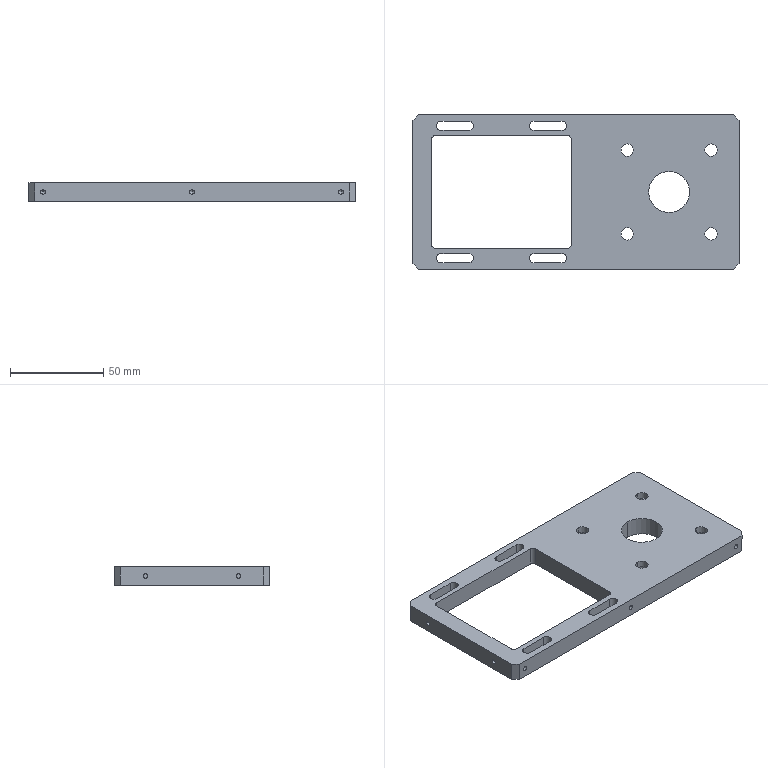Part | SolidWorks | features BaseBody 1 | 1 solid | 88 faces | box 175 x 83 x 10 mm | volume 88673 mm3 | cylinder 50 | plane 26 | cone 12 | commonest cylinder face diameters 2.5 x20 5 x8 6.6 x8 11 x8 4 x4 22 x2